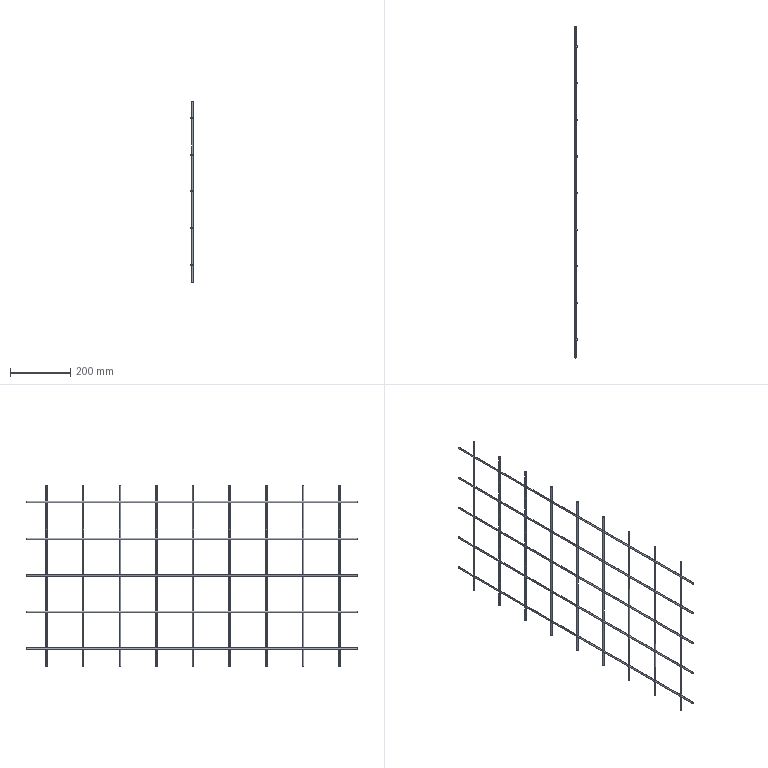Part | 1 solid | 56 faces | box 8 x 1105 x 606 mm | volume 214451 mm3 | cylinder 28 | plane 28 | commonest cylinder face diameters 5 x28